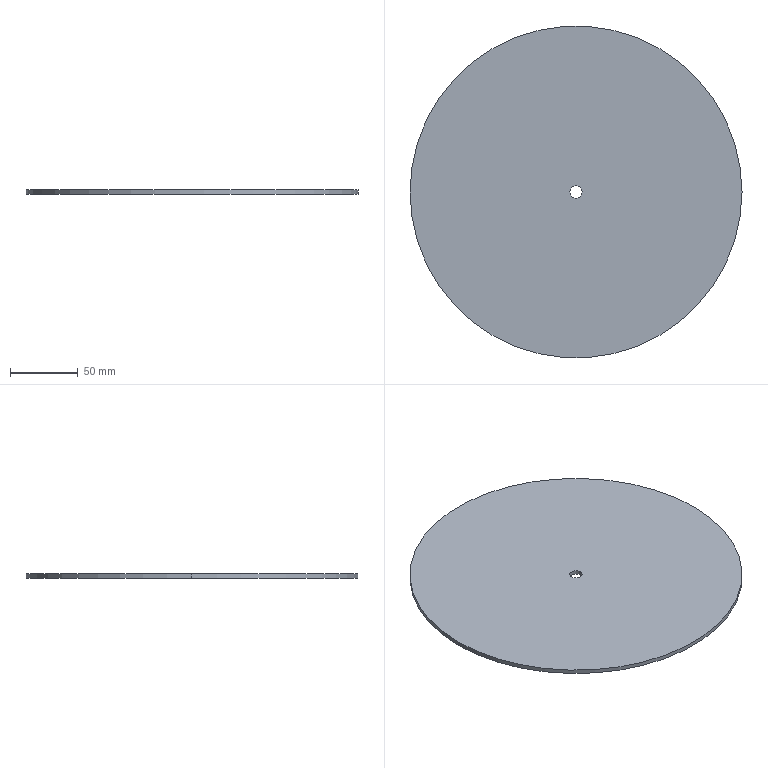Part | SolidWorks | features Extrusion 1 | 1 solid | 6 faces | box 244.5 x 244.5 x 3 mm | volume 140663 mm3 | cylinder 4 | plane 2 | commonest cylinder face diameters 9 x2 244.5 x2
STEP:
#1=CARTESIAN_POINT('',(-4.5,0.,3.));
#2=VERTEX_POINT('',#1);
#3=CARTESIAN_POINT('',(4.5,0.,3.));
#4=VERTEX_POINT('',#3);
#5=CARTESIAN_POINT('',(0.,0.,3.));
#6=DIRECTION('',(0.,0.,1.));
#7=DIRECTION('',(1.,0.,0.));
#8=AXIS2_PLACEMENT_3D('',#5,#6,#7);
#9=CIRCLE('',#8,4.5);
#10=EDGE_CURVE('',#2,#4,#9,.T.);
#11=ORIENTED_EDGE('',*,*,#10,.T.);
#12=CARTESIAN_POINT('',(4.5,0.,0.));
#13=VERTEX_POINT('',#12);
#14=CARTESIAN_POINT('',(4.5,0.,3.));
#15=DIRECTION('',(0.,0.,-1.));
#16=VECTOR('',#15,1000.);
#17=LINE('',#14,#16);
#18=EDGE_CURVE('',#4,#13,#17,.T.);
#19=ORIENTED_EDGE('',*,*,#18,.T.);
#20=CARTESIAN_POINT('',(-4.5,0.,0.));
#21=VERTEX_POINT('',#20);
#22=CARTESIAN_POINT('',(0.,0.,0.));
#23=DIRECTION('',(0.,0.,1.));
#24=DIRECTION('',(1.,0.,0.));
#25=AXIS2_PLACEMENT_3D('',#22,#23,#24);
#26=CIRCLE('',#25,4.5);
#27=EDGE_CURVE('',#21,#13,#26,.T.);
#28=ORIENTED_EDGE('',*,*,#27,.F.);
#29=CARTESIAN_POINT('',(-4.5,0.,3.));
#30=DIRECTION('',(0.,0.,-1.));
#31=VECTOR('',#30,1000.);
#32=LINE('',#29,#31);
#33=EDGE_CURVE('',#2,#21,#32,.T.);
#34=ORIENTED_EDGE('',*,*,#33,.F.);
#35=EDGE_LOOP('',(#11,#19,#28,#34));
#36=FACE_OUTER_BOUND('',#35,.T.);
#37=CARTESIAN_POINT('',(0.,0.,3.));
#38=DIRECTION('',(0.,0.,-1.));
#39=DIRECTION('',(-1.,0.,0.));
#40=AXIS2_PLACEMENT_3D('',#37,#38,#39);
#41=CYLINDRICAL_SURFACE('',#40,4.5);
#42=ADVANCED_FACE('',(#36),#41,.F.);
#43=CARTESIAN_POINT('',(122.25,0.,3.));
#44=VERTEX_POINT('',#43);
#45=CARTESIAN_POINT('',(-122.25,0.,3.));
#46=VERTEX_POINT('',#45);
#47=CARTESIAN_POINT('',(0.,0.,3.));
#48=DIRECTION('',(0.,0.,1.));
#49=DIRECTION('',(1.,0.,0.));
#50=AXIS2_PLACEMENT_3D('',#47,#48,#49);
#51=CIRCLE('',#50,122.25);
#52=EDGE_CURVE('',#44,#46,#51,.T.);
#53=ORIENTED_EDGE('',*,*,#52,.F.);
#54=CARTESIAN_POINT('',(122.25,0.,0.));
#55=VERTEX_POINT('',#54);
#56=CARTESIAN_POINT('',(122.25,0.,3.));
#57=DIRECTION('',(0.,0.,-1.));
#58=VECTOR('',#57,1000.);
#59=LINE('',#56,#58);
#60=EDGE_CURVE('',#44,#55,#59,.T.);
#61=ORIENTED_EDGE('',*,*,#60,.T.);
#62=CARTESIAN_POINT('',(-122.25,0.,0.));
#63=VERTEX_POINT('',#62);
#64=CARTESIAN_POINT('',(0.,0.,0.));
#65=DIRECTION('',(0.,0.,1.));
#66=DIRECTION('',(1.,0.,0.));
#67=AXIS2_PLACEMENT_3D('',#64,#65,#66);
#68=CIRCLE('',#67,122.25);
#69=EDGE_CURVE('',#55,#63,#68,.T.);
#70=ORIENTED_EDGE('',*,*,#69,.T.);
#71=CARTESIAN_POINT('',(-122.25,0.,3.));
#72=DIRECTION('',(0.,0.,-1.));
#73=VECTOR('',#72,1000.);
#74=LINE('',#71,#73);
#75=EDGE_CURVE('',#46,#63,#74,.T.);
#76=ORIENTED_EDGE('',*,*,#75,.F.);
#77=EDGE_LOOP('',(#53,#61,#70,#76));
#78=FACE_OUTER_BOUND('',#77,.T.);
#79=CARTESIAN_POINT('',(0.,0.,3.));
#80=DIRECTION('',(0.,0.,-1.));
#81=DIRECTION('',(-1.,0.,0.));
#82=AXIS2_PLACEMENT_3D('',#79,#80,#81);
#83=CYLINDRICAL_SURFACE('',#82,122.25);
#84=ADVANCED_FACE('',(#78),#83,.T.);
#85=CARTESIAN_POINT('',(0.,0.,3.));
#86=DIRECTION('',(0.,0.,1.));
#87=DIRECTION('',(1.,0.,0.));
#88=AXIS2_PLACEMENT_3D('',#85,#86,#87);
#89=CIRCLE('',#88,122.25);
#90=EDGE_CURVE('',#46,#44,#89,.T.);
#91=ORIENTED_EDGE('',*,*,#90,.T.);
#92=ORIENTED_EDGE('',*,*,#52,.T.);
#93=EDGE_LOOP('',(#91,#92));
#94=FACE_OUTER_BOUND('',#93,.T.);
#95=ORIENTED_EDGE('',*,*,#10,.F.);
#96=CARTESIAN_POINT('',(0.,0.,3.));
#97=DIRECTION('',(0.,0.,1.));
#98=DIRECTION('',(1.,0.,0.));
#99=AXIS2_PLACEMENT_3D('',#96,#97,#98);
#100=CIRCLE('',#99,4.5);
#101=EDGE_CURVE('',#4,#2,#100,.T.);
#102=ORIENTED_EDGE('',*,*,#101,.F.);
#103=EDGE_LOOP('',(#95,#102));
#104=FACE_BOUND('',#103,.T.);
#105=CARTESIAN_POINT('',(0.,0.,3.));
#106=DIRECTION('',(0.,0.,1.));
#107=DIRECTION('',(1.,0.,0.));
#108=AXIS2_PLACEMENT_3D('',#105,#106,#107);
#109=PLANE('',#108);
#110=ADVANCED_FACE('',(#94,#104),#109,.T.);
#111=CARTESIAN_POINT('',(0.,0.,0.));
#112=DIRECTION('',(0.,0.,1.));
#113=DIRECTION('',(1.,0.,0.));
#114=AXIS2_PLACEMENT_3D('',#111,#112,#113);
#115=CIRCLE('',#114,122.25);
#116=EDGE_CURVE('',#63,#55,#115,.T.);
#117=ORIENTED_EDGE('',*,*,#116,.F.);
#118=ORIENTED_EDGE('',*,*,#69,.F.);
#119=EDGE_LOOP('',(#117,#118));
#120=FACE_OUTER_BOUND('',#119,.T.);
#121=ORIENTED_EDGE('',*,*,#27,.T.);
#122=CARTESIAN_POINT('',(0.,0.,0.));
#123=DIRECTION('',(0.,0.,1.));
#124=DIRECTION('',(1.,0.,0.));
#125=AXIS2_PLACEMENT_3D('',#122,#123,#124);
#126=CIRCLE('',#125,4.5);
#127=EDGE_CURVE('',#13,#21,#126,.T.);
#128=ORIENTED_EDGE('',*,*,#127,.T.);
#129=EDGE_LOOP('',(#121,#128));
#130=FACE_BOUND('',#129,.T.);
#131=CARTESIAN_POINT('',(0.,0.,0.));
#132=DIRECTION('',(0.,0.,1.));
#133=DIRECTION('',(1.,0.,0.));
#134=AXIS2_PLACEMENT_3D('',#131,#132,#133);
#135=PLANE('',#134);
#136=ADVANCED_FACE('',(#120,#130),#135,.F.);
#137=ORIENTED_EDGE('',*,*,#60,.F.);
#138=ORIENTED_EDGE('',*,*,#90,.F.);
#139=ORIENTED_EDGE('',*,*,#75,.T.);
#140=ORIENTED_EDGE('',*,*,#116,.T.);
#141=EDGE_LOOP('',(#137,#138,#139,#140));
#142=FACE_OUTER_BOUND('',#141,.T.);
#143=CARTESIAN_POINT('',(0.,0.,3.));
#144=DIRECTION('',(0.,0.,-1.));
#145=DIRECTION('',(-1.,0.,0.));
#146=AXIS2_PLACEMENT_3D('',#143,#144,#145);
#147=CYLINDRICAL_SURFACE('',#146,122.25);
#148=ADVANCED_FACE('',(#142),#147,.T.);
#149=ORIENTED_EDGE('',*,*,#18,.F.);
#150=ORIENTED_EDGE('',*,*,#101,.T.);
#151=ORIENTED_EDGE('',*,*,#33,.T.);
#152=ORIENTED_EDGE('',*,*,#127,.F.);
#153=EDGE_LOOP('',(#149,#150,#151,#152));
#154=FACE_OUTER_BOUND('',#153,.T.);
#155=CARTESIAN_POINT('',(0.,0.,3.));
#156=DIRECTION('',(0.,0.,-1.));
#157=DIRECTION('',(-1.,0.,0.));
#158=AXIS2_PLACEMENT_3D('',#155,#156,#157);
#159=CYLINDRICAL_SURFACE('',#158,4.5);
#160=ADVANCED_FACE('',(#154),#159,.F.);
#161=CLOSED_SHELL('',(#42,#84,#110,#136,#148,#160));
#162=MANIFOLD_SOLID_BREP('',#161);
#163=CARTESIAN_POINT('',(0.,0.,0.));
#164=DIRECTION('',(0.,0.,1.));
#165=DIRECTION('',(1.,0.,0.));
#166=AXIS2_PLACEMENT_3D('',#163,#164,#165);
#167=(LENGTH_UNIT()NAMED_UNIT(*)SI_UNIT(.MILLI.,.METRE.));
#168=UNCERTAINTY_MEASURE_WITH_UNIT(LENGTH_MEASURE(0.00001),#167,'','');
#169=(NAMED_UNIT(*)PLANE_ANGLE_UNIT()SI_UNIT($,.RADIAN.));
#170=(NAMED_UNIT(*)SI_UNIT($,.STERADIAN.)SOLID_ANGLE_UNIT());
#171=(GEOMETRIC_REPRESENTATION_CONTEXT(3)GLOBAL_UNCERTAINTY_ASSIGNED_CONTEXT((#168))GLOBAL_UNIT_ASSIGNED_CONTEXT((#167,#169,#170))REPRESENTATION_CONTEXT('',''));
#172=ADVANCED_BREP_SHAPE_REPRESENTATION('',(#162,#166),#171);